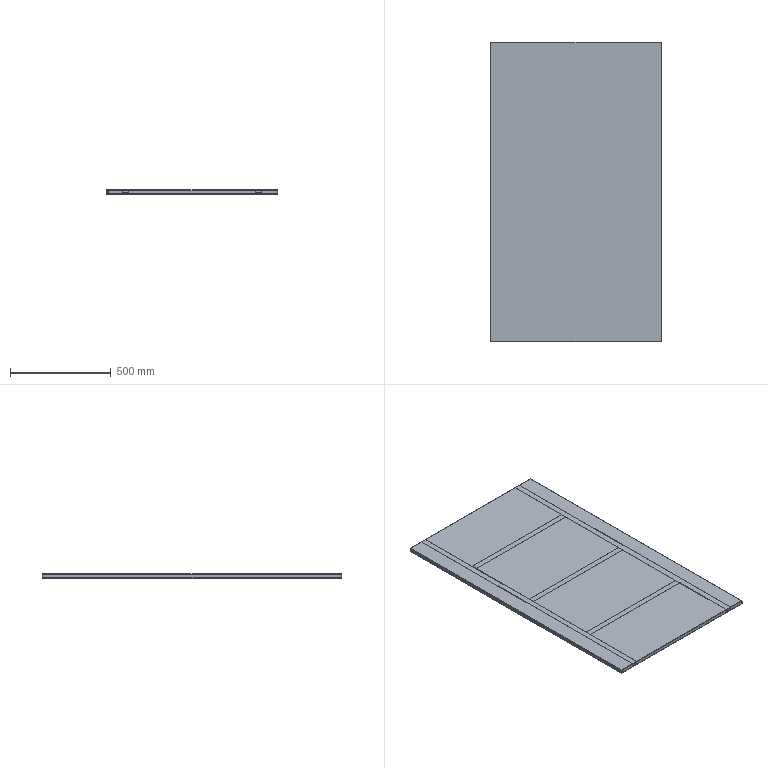Part | SolidWorks | features BaseBody 6 | 6 solids | 124 faces | box 848 x 1486 x 20 mm | volume 1659085 mm3 | plane 88 | cylinder 20 | spline 16 | commonest cylinder face diameters 2 x8 4 x8 8 x4